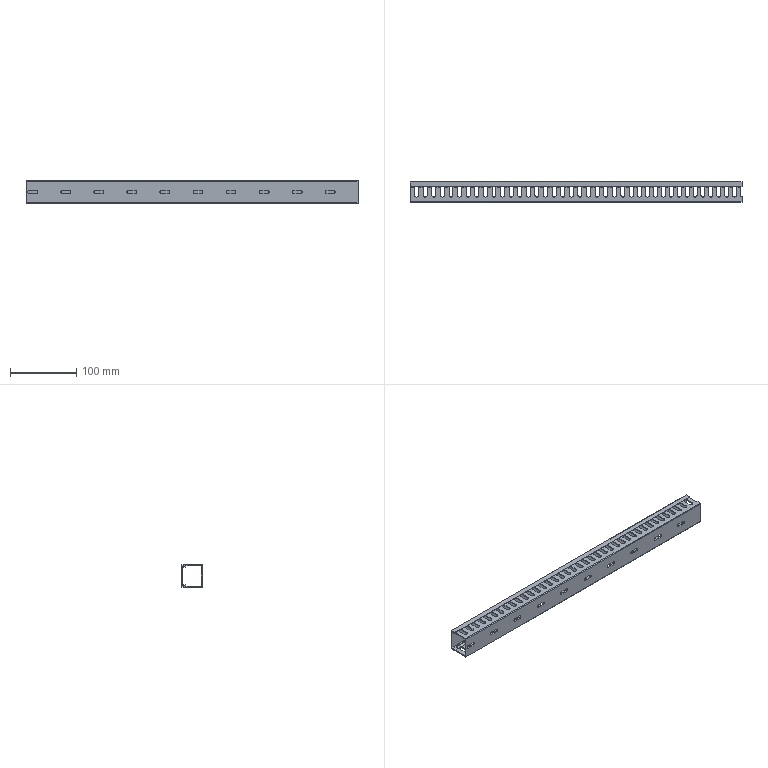Part | SolidWorks | features BaseBody 2, ICE 1 | 2 solids | 708 faces | box 502 x 31.5 x 34 mm | volume 88043 mm3 | plane 600 | cylinder 108 | commonest cylinder face diameters 6 x80 5 x20 1 x4 0.2 x2 2 x2